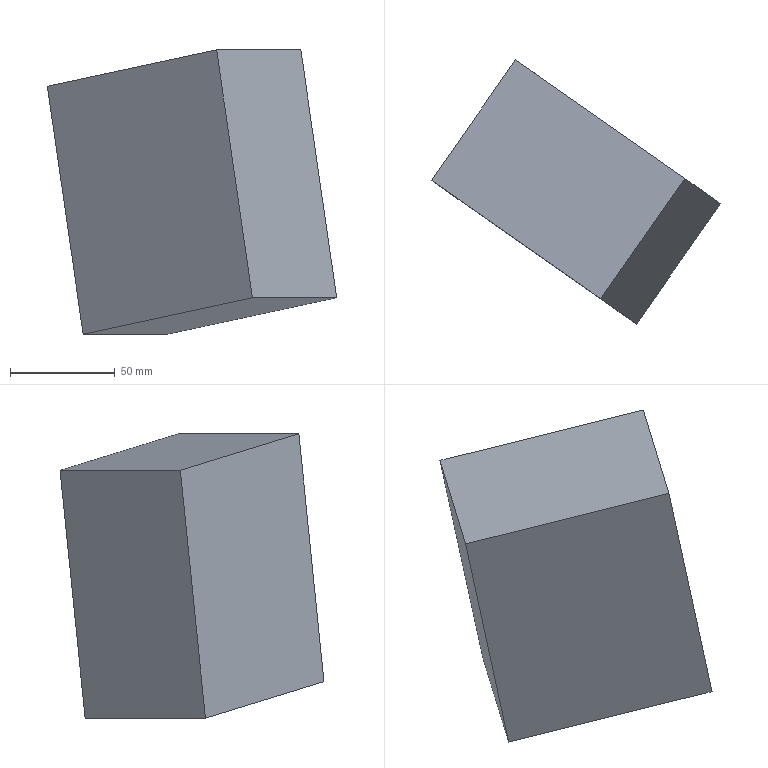Part | NX | features solid 2 | 1 solid | 6 faces | box 137.89 x 125.779 x 135.542 mm | volume 840000 mm3 | plane 6
STEP:
#1=CARTESIAN_POINT('',(-378.379,94.035,-114.723));
#2=VERTEX_POINT('',#1);
#3=CARTESIAN_POINT('',(-459.049,150.521,-132.088));
#4=VERTEX_POINT('',#3);
#5=CARTESIAN_POINT('',(-394.513,105.332,-118.196));
#6=DIRECTION('',(-0.8067,0.5649,-0.1736));
#7=VECTOR('',#6,1000.);
#8=LINE('',#5,#7);
#9=EDGE_CURVE('',#2,#4,#8,.T.);
#10=ORIENTED_EDGE('',*,*,#9,.T.);
#11=CARTESIAN_POINT('',(-499.2,93.181,-132.088));
#12=VERTEX_POINT('',#11);
#13=CARTESIAN_POINT('',(-499.2,93.181,-132.088));
#14=DIRECTION('',(0.5736,0.8192,0.));
#15=VECTOR('',#14,1000.);
#16=LINE('',#13,#15);
#17=EDGE_CURVE('',#12,#4,#16,.T.);
#18=ORIENTED_EDGE('',*,*,#17,.F.);
#19=CARTESIAN_POINT('',(-418.529,36.695,-114.723));
#20=VERTEX_POINT('',#19);
#21=CARTESIAN_POINT('',(-434.663,47.992,-118.196));
#22=DIRECTION('',(-0.8067,0.5649,-0.1736));
#23=VECTOR('',#22,1000.);
#24=LINE('',#21,#23);
#25=EDGE_CURVE('',#20,#12,#24,.T.);
#26=ORIENTED_EDGE('',*,*,#25,.F.);
#27=CARTESIAN_POINT('',(-418.529,36.695,-114.723));
#28=DIRECTION('',(0.5736,0.8192,0.));
#29=VECTOR('',#28,1000.);
#30=LINE('',#27,#29);
#31=EDGE_CURVE('',#20,#2,#30,.T.);
#32=ORIENTED_EDGE('',*,*,#31,.T.);
#33=EDGE_LOOP('',(#10,#18,#26,#32));
#34=FACE_BOUND('',#33,.T.);
#35=CARTESIAN_POINT('',(-434.663,47.992,-118.196));
#36=DIRECTION('',(0.1422,-0.0996,-0.9848));
#37=DIRECTION('',(-0.8067,0.5649,-0.1736));
#38=AXIS2_PLACEMENT_3D('',#35,#36,#37);
#39=PLANE('',#38);
#40=ADVANCED_FACE('',(#34),#39,.F.);
#41=ORIENTED_EDGE('',*,*,#17,.T.);
#42=CARTESIAN_POINT('',(-441.98,138.569,-250.264));
#43=VERTEX_POINT('',#42);
#44=CARTESIAN_POINT('',(-458.338,150.023,-137.012));
#45=DIRECTION('',(-0.1422,0.0996,0.9848));
#46=VECTOR('',#45,1000.);
#47=LINE('',#44,#46);
#48=EDGE_CURVE('',#4,#43,#47,.F.);
#49=ORIENTED_EDGE('',*,*,#48,.T.);
#50=CARTESIAN_POINT('',(-482.131,81.229,-250.264));
#51=VERTEX_POINT('',#50);
#52=CARTESIAN_POINT('',(-482.131,81.229,-250.264));
#53=DIRECTION('',(-0.5736,-0.8192,0.));
#54=VECTOR('',#53,1000.);
#55=LINE('',#52,#54);
#56=EDGE_CURVE('',#51,#43,#55,.F.);
#57=ORIENTED_EDGE('',*,*,#56,.F.);
#58=CARTESIAN_POINT('',(-498.489,92.683,-137.012));
#59=DIRECTION('',(0.1422,-0.0996,-0.9848));
#60=VECTOR('',#59,1000.);
#61=LINE('',#58,#60);
#62=EDGE_CURVE('',#12,#51,#61,.T.);
#63=ORIENTED_EDGE('',*,*,#62,.F.);
#64=EDGE_LOOP('',(#41,#49,#57,#63));
#65=FACE_BOUND('',#64,.T.);
#66=CARTESIAN_POINT('',(-498.489,92.683,-137.012));
#67=DIRECTION('',(0.8067,-0.5649,0.1736));
#68=DIRECTION('',(0.1422,-0.0996,-0.9848));
#69=AXIS2_PLACEMENT_3D('',#66,#67,#68);
#70=PLANE('',#69);
#71=ADVANCED_FACE('',(#65),#70,.F.);
#72=ORIENTED_EDGE('',*,*,#56,.T.);
#73=CARTESIAN_POINT('',(-361.309,82.083,-232.9));
#74=VERTEX_POINT('',#73);
#75=CARTESIAN_POINT('',(-377.444,93.38,-236.373));
#76=DIRECTION('',(0.8067,-0.5649,0.1736));
#77=VECTOR('',#76,1000.);
#78=LINE('',#75,#77);
#79=EDGE_CURVE('',#74,#43,#78,.F.);
#80=ORIENTED_EDGE('',*,*,#79,.F.);
#81=CARTESIAN_POINT('',(-401.46,24.742,-232.9));
#82=VERTEX_POINT('',#81);
#83=CARTESIAN_POINT('',(-401.46,24.742,-232.9));
#84=DIRECTION('',(-0.5736,-0.8192,0.));
#85=VECTOR('',#84,1000.);
#86=LINE('',#83,#85);
#87=EDGE_CURVE('',#82,#74,#86,.F.);
#88=ORIENTED_EDGE('',*,*,#87,.F.);
#89=CARTESIAN_POINT('',(-417.594,36.04,-236.373));
#90=DIRECTION('',(0.8067,-0.5649,0.1736));
#91=VECTOR('',#90,1000.);
#92=LINE('',#89,#91);
#93=EDGE_CURVE('',#82,#51,#92,.F.);
#94=ORIENTED_EDGE('',*,*,#93,.T.);
#95=EDGE_LOOP('',(#72,#80,#88,#94));
#96=FACE_BOUND('',#95,.T.);
#97=CARTESIAN_POINT('',(-417.594,36.04,-236.373));
#98=DIRECTION('',(0.1422,-0.0996,-0.9848));
#99=DIRECTION('',(-0.8067,0.5649,-0.1736));
#100=AXIS2_PLACEMENT_3D('',#97,#98,#99);
#101=PLANE('',#100);
#102=ADVANCED_FACE('',(#96),#101,.T.);
#103=ORIENTED_EDGE('',*,*,#79,.T.);
#104=ORIENTED_EDGE('',*,*,#48,.F.);
#105=ORIENTED_EDGE('',*,*,#9,.F.);
#106=CARTESIAN_POINT('',(-377.668,93.537,-119.647));
#107=DIRECTION('',(0.1422,-0.0996,-0.9848));
#108=VECTOR('',#107,1000.);
#109=LINE('',#106,#108);
#110=EDGE_CURVE('',#2,#74,#109,.T.);
#111=ORIENTED_EDGE('',*,*,#110,.T.);
#112=EDGE_LOOP('',(#103,#104,#105,#111));
#113=FACE_BOUND('',#112,.T.);
#114=CARTESIAN_POINT('',(-393.802,104.834,-123.12));
#115=DIRECTION('',(0.5736,0.8192,0.));
#116=DIRECTION('',(-0.8192,0.5736,0.));
#117=AXIS2_PLACEMENT_3D('',#114,#115,#116);
#118=PLANE('',#117);
#119=ADVANCED_FACE('',(#113),#118,.T.);
#120=ORIENTED_EDGE('',*,*,#25,.T.);
#121=ORIENTED_EDGE('',*,*,#62,.T.);
#122=ORIENTED_EDGE('',*,*,#93,.F.);
#123=CARTESIAN_POINT('',(-417.818,36.197,-119.647));
#124=DIRECTION('',(-0.1422,0.0996,0.9848));
#125=VECTOR('',#124,1000.);
#126=LINE('',#123,#125);
#127=EDGE_CURVE('',#82,#20,#126,.T.);
#128=ORIENTED_EDGE('',*,*,#127,.T.);
#129=EDGE_LOOP('',(#120,#121,#122,#128));
#130=FACE_BOUND('',#129,.T.);
#131=CARTESIAN_POINT('',(-433.952,47.494,-123.12));
#132=DIRECTION('',(0.5736,0.8192,0.));
#133=DIRECTION('',(-0.8192,0.5736,0.));
#134=AXIS2_PLACEMENT_3D('',#131,#132,#133);
#135=PLANE('',#134);
#136=ADVANCED_FACE('',(#130),#135,.F.);
#137=ORIENTED_EDGE('',*,*,#31,.F.);
#138=ORIENTED_EDGE('',*,*,#127,.F.);
#139=ORIENTED_EDGE('',*,*,#87,.T.);
#140=ORIENTED_EDGE('',*,*,#110,.F.);
#141=EDGE_LOOP('',(#137,#138,#139,#140));
#142=FACE_BOUND('',#141,.T.);
#143=CARTESIAN_POINT('',(-417.818,36.197,-119.647));
#144=DIRECTION('',(0.8067,-0.5649,0.1736));
#145=DIRECTION('',(0.1422,-0.0996,-0.9848));
#146=AXIS2_PLACEMENT_3D('',#143,#144,#145);
#147=PLANE('',#146);
#148=ADVANCED_FACE('',(#142),#147,.T.);
#149=CLOSED_SHELL('',(#40,#71,#102,#119,#136,#148));
#150=MANIFOLD_SOLID_BREP('',#149);
#151=(LENGTH_UNIT()NAMED_UNIT(*)SI_UNIT(.MILLI.,.METRE.));
#152=UNCERTAINTY_MEASURE_WITH_UNIT(LENGTH_MEASURE(0.00001),#151,'','');
#153=(NAMED_UNIT(*)PLANE_ANGLE_UNIT()SI_UNIT($,.RADIAN.));
#154=(NAMED_UNIT(*)SI_UNIT($,.STERADIAN.)SOLID_ANGLE_UNIT());
#155=(GEOMETRIC_REPRESENTATION_CONTEXT(3)GLOBAL_UNCERTAINTY_ASSIGNED_CONTEXT((#152))GLOBAL_UNIT_ASSIGNED_CONTEXT((#151,#153,#154))REPRESENTATION_CONTEXT('',''));
#156=ADVANCED_BREP_SHAPE_REPRESENTATION('',(#150),#155);